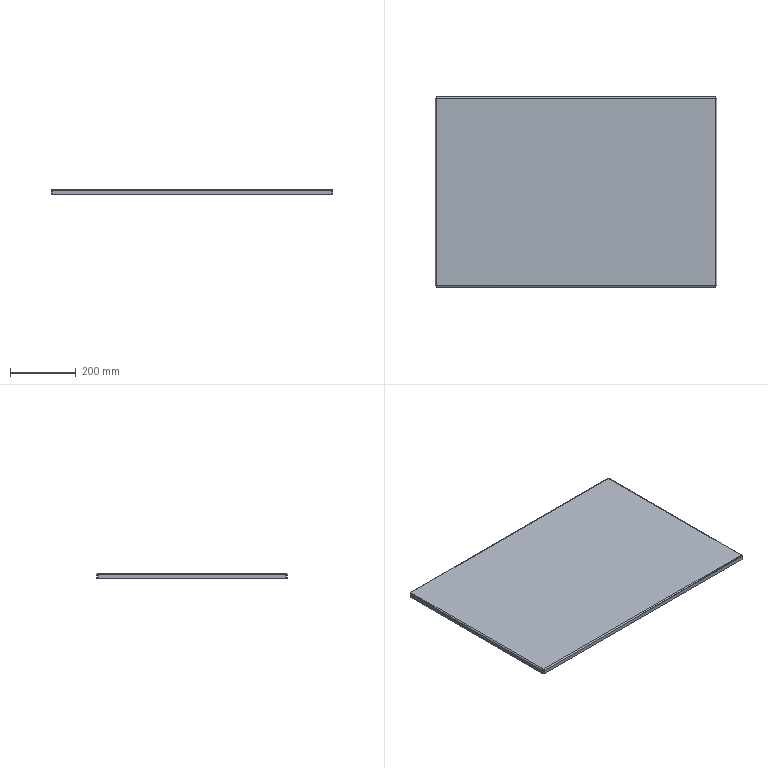Part | STEP file | MYT-A01-P36 | 1 solid | 38 faces | box 860 x 580 x 15 mm | volume 1590637 mm3 | plane 22 | spline 8 | cylinder 8 | commonest cylinder face diameters 1.473 x4 7.473 x4
STEP:
#1=CARTESIAN_POINT('',(-426.263,-286.263,-3.));
#2=VERTEX_POINT('',#1);
#3=CARTESIAN_POINT('',(426.263,-286.263,-3.));
#4=VERTEX_POINT('',#3);
#5=CARTESIAN_POINT('',(-426.293,-286.263,-3.));
#6=DIRECTION('',(1.,0.,0.));
#7=VECTOR('',#6,1000.);
#8=LINE('',#5,#7);
#9=EDGE_CURVE('',#2,#4,#8,.T.);
#10=ORIENTED_EDGE('',*,*,#9,.F.);
#11=CARTESIAN_POINT('',(-426.263,286.263,-3.));
#12=VERTEX_POINT('',#11);
#13=CARTESIAN_POINT('',(-426.263,286.293,-3.));
#14=DIRECTION('',(0.,-1.,0.));
#15=VECTOR('',#14,1000.);
#16=LINE('',#13,#15);
#17=EDGE_CURVE('',#12,#2,#16,.T.);
#18=ORIENTED_EDGE('',*,*,#17,.F.);
#19=CARTESIAN_POINT('',(426.263,286.263,-3.));
#20=VERTEX_POINT('',#19);
#21=CARTESIAN_POINT('',(426.293,286.263,-3.));
#22=DIRECTION('',(-1.,0.,0.));
#23=VECTOR('',#22,1000.);
#24=LINE('',#21,#23);
#25=EDGE_CURVE('',#20,#12,#24,.T.);
#26=ORIENTED_EDGE('',*,*,#25,.F.);
#27=CARTESIAN_POINT('',(426.263,-286.293,-3.));
#28=DIRECTION('',(0.,1.,0.));
#29=VECTOR('',#28,1000.);
#30=LINE('',#27,#29);
#31=EDGE_CURVE('',#4,#20,#30,.T.);
#32=ORIENTED_EDGE('',*,*,#31,.F.);
#33=EDGE_LOOP('',(#10,#18,#26,#32));
#34=FACE_OUTER_BOUND('',#33,.T.);
#35=CARTESIAN_POINT('',(0.,0.,-3.));
#36=DIRECTION('',(0.,0.,1.));
#37=DIRECTION('',(1.,0.,0.));
#38=AXIS2_PLACEMENT_3D('',#35,#36,#37);
#39=PLANE('',#38);
#40=ADVANCED_FACE('',(#34),#39,.F.);
#41=CARTESIAN_POINT('',(-426.263,286.263,0.));
#42=VERTEX_POINT('',#41);
#43=CARTESIAN_POINT('',(-426.263,-286.263,0.));
#44=VERTEX_POINT('',#43);
#45=CARTESIAN_POINT('',(-426.263,286.293,0.));
#46=DIRECTION('',(0.,-1.,0.));
#47=VECTOR('',#46,1000.);
#48=LINE('',#45,#47);
#49=EDGE_CURVE('',#42,#44,#48,.T.);
#50=ORIENTED_EDGE('',*,*,#49,.T.);
#51=CARTESIAN_POINT('',(426.263,-286.263,0.));
#52=VERTEX_POINT('',#51);
#53=CARTESIAN_POINT('',(-426.293,-286.263,0.));
#54=DIRECTION('',(1.,0.,0.));
#55=VECTOR('',#54,1000.);
#56=LINE('',#53,#55);
#57=EDGE_CURVE('',#44,#52,#56,.T.);
#58=ORIENTED_EDGE('',*,*,#57,.T.);
#59=CARTESIAN_POINT('',(426.263,286.263,0.));
#60=VERTEX_POINT('',#59);
#61=CARTESIAN_POINT('',(426.263,-286.293,0.));
#62=DIRECTION('',(0.,1.,0.));
#63=VECTOR('',#62,1000.);
#64=LINE('',#61,#63);
#65=EDGE_CURVE('',#52,#60,#64,.T.);
#66=ORIENTED_EDGE('',*,*,#65,.T.);
#67=CARTESIAN_POINT('',(426.293,286.263,0.));
#68=DIRECTION('',(-1.,0.,0.));
#69=VECTOR('',#68,1000.);
#70=LINE('',#67,#69);
#71=EDGE_CURVE('',#60,#42,#70,.T.);
#72=ORIENTED_EDGE('',*,*,#71,.T.);
#73=EDGE_LOOP('',(#50,#58,#66,#72));
#74=FACE_OUTER_BOUND('',#73,.T.);
#75=CARTESIAN_POINT('',(0.,0.,0.));
#76=DIRECTION('',(0.,0.,1.));
#77=DIRECTION('',(1.,0.,0.));
#78=AXIS2_PLACEMENT_3D('',#75,#76,#77);
#79=PLANE('',#78);
#80=ADVANCED_FACE('',(#74),#79,.T.);
#81=CARTESIAN_POINT('',(430.,286.293,-3.737));
#82=VERTEX_POINT('',#81);
#83=CARTESIAN_POINT('',(427.,286.293,-3.737));
#84=VERTEX_POINT('',#83);
#85=CARTESIAN_POINT('',(427.,286.293,-3.737));
#86=DIRECTION('',(-1.,0.,0.));
#87=VECTOR('',#86,1000.);
#88=LINE('',#85,#87);
#89=EDGE_CURVE('',#82,#84,#88,.T.);
#90=ORIENTED_EDGE('',*,*,#89,.T.);
#91=CARTESIAN_POINT('',(426.263,286.263,-3.));
#92=CARTESIAN_POINT('',(426.456,286.268,-3.));
#93=CARTESIAN_POINT('',(426.648,286.273,-3.079));
#94=CARTESIAN_POINT('',(426.921,286.283,-3.352));
#95=CARTESIAN_POINT('',(427.,286.288,-3.544));
#96=CARTESIAN_POINT('',(427.,286.293,-3.737));
#97=B_SPLINE_CURVE_WITH_KNOTS('',3,(#91,#92,#93,#94,#95,#96),.UNSPECIFIED.,.F.,.F.,(4,2,4),(0.,0.5,1.),.UNSPECIFIED.);
#98=EDGE_CURVE('',#20,#84,#97,.T.);
#99=ORIENTED_EDGE('',*,*,#98,.F.);
#100=CARTESIAN_POINT('',(426.263,286.263,-3.));
#101=DIRECTION('',(0.,0.,1.));
#102=VECTOR('',#101,1000.);
#103=LINE('',#100,#102);
#104=EDGE_CURVE('',#20,#60,#103,.T.);
#105=ORIENTED_EDGE('',*,*,#104,.T.);
#106=CARTESIAN_POINT('',(426.263,286.263,0.));
#107=CARTESIAN_POINT('',(426.753,286.266,0.));
#108=CARTESIAN_POINT('',(427.241,286.268,-0.09725));
#109=CARTESIAN_POINT('',(428.145,286.273,-0.4716));
#110=CARTESIAN_POINT('',(428.56,286.276,-0.7486));
#111=CARTESIAN_POINT('',(429.251,286.281,-1.44));
#112=CARTESIAN_POINT('',(429.528,286.283,-1.855));
#113=CARTESIAN_POINT('',(429.903,286.288,-2.759));
#114=CARTESIAN_POINT('',(430.,286.29,-3.247));
#115=CARTESIAN_POINT('',(430.,286.293,-3.737));
#116=B_SPLINE_CURVE_WITH_KNOTS('',3,(#106,#107,#108,#109,#110,#111,#112,#113,#114,#115),.UNSPECIFIED.,.F.,.F.,(4,2,2,2,4),(0.,0.25,0.5,0.75,1.),.UNSPECIFIED.);
#117=EDGE_CURVE('',#60,#82,#116,.T.);
#118=ORIENTED_EDGE('',*,*,#117,.T.);
#119=EDGE_LOOP('',(#90,#99,#105,#118));
#120=FACE_OUTER_BOUND('',#119,.T.);
#121=CARTESIAN_POINT('',(426.263,286.263,0.03));
#122=CARTESIAN_POINT('',(426.757,286.266,0.03));
#123=CARTESIAN_POINT('',(427.249,286.268,-0.06803));
#124=CARTESIAN_POINT('',(428.16,286.273,-0.4454));
#125=CARTESIAN_POINT('',(428.578,286.276,-0.7246));
#126=CARTESIAN_POINT('',(429.275,286.281,-1.422));
#127=CARTESIAN_POINT('',(429.555,286.283,-1.84));
#128=CARTESIAN_POINT('',(429.932,286.288,-2.751));
#129=CARTESIAN_POINT('',(430.03,286.29,-3.243));
#130=CARTESIAN_POINT('',(430.03,286.293,-3.737));
#131=CARTESIAN_POINT('',(426.263,286.263,0.));
#132=CARTESIAN_POINT('',(426.753,286.266,0.));
#133=CARTESIAN_POINT('',(427.241,286.268,-0.09725));
#134=CARTESIAN_POINT('',(428.145,286.273,-0.4716));
#135=CARTESIAN_POINT('',(428.56,286.276,-0.7486));
#136=CARTESIAN_POINT('',(429.251,286.281,-1.44));
#137=CARTESIAN_POINT('',(429.528,286.283,-1.855));
#138=CARTESIAN_POINT('',(429.903,286.288,-2.759));
#139=CARTESIAN_POINT('',(430.,286.29,-3.247));
#140=CARTESIAN_POINT('',(430.,286.293,-3.737));
#141=CARTESIAN_POINT('',(426.263,286.263,-3.));
#142=CARTESIAN_POINT('',(426.36,286.266,-3.));
#143=CARTESIAN_POINT('',(426.456,286.268,-3.019));
#144=CARTESIAN_POINT('',(426.634,286.273,-3.093));
#145=CARTESIAN_POINT('',(426.716,286.276,-3.148));
#146=CARTESIAN_POINT('',(426.852,286.281,-3.284));
#147=CARTESIAN_POINT('',(426.907,286.283,-3.366));
#148=CARTESIAN_POINT('',(426.981,286.288,-3.544));
#149=CARTESIAN_POINT('',(427.,286.29,-3.64));
#150=CARTESIAN_POINT('',(427.,286.293,-3.737));
#151=CARTESIAN_POINT('',(426.263,286.263,-3.03));
#152=CARTESIAN_POINT('',(426.356,286.266,-3.03));
#153=CARTESIAN_POINT('',(426.448,286.268,-3.049));
#154=CARTESIAN_POINT('',(426.619,286.273,-3.119));
#155=CARTESIAN_POINT('',(426.697,286.276,-3.172));
#156=CARTESIAN_POINT('',(426.828,286.281,-3.303));
#157=CARTESIAN_POINT('',(426.881,286.283,-3.381));
#158=CARTESIAN_POINT('',(426.951,286.288,-3.552));
#159=CARTESIAN_POINT('',(426.97,286.29,-3.644));
#160=CARTESIAN_POINT('',(426.97,286.293,-3.737));
#161=B_SPLINE_SURFACE_WITH_KNOTS('',1,3,((#121,#122,#123,#124,#125,#126,#127,#128,#129,#130),(#131,#132,#133,#134,#135,#136,#137,#138,#139,#140),(#141,#142,#143,#144,#145,#146,#147,#148,#149,#150),(#151,#152,#153,#154,#155,#156,#157,#158,#159,#160)),.UNSPECIFIED.,.F.,.F.,.F.,(2,1,1,2),(4,2,2,2,4),(-0.01,0.,1.,1.01),(0.,0.25,0.5,0.75,1.),.UNSPECIFIED.);
#162=ADVANCED_FACE('',(#120),#161,.F.);
#163=CARTESIAN_POINT('',(427.,-286.293,-3.737));
#164=VERTEX_POINT('',#163);
#165=CARTESIAN_POINT('',(427.,-286.293,-3.737));
#166=CARTESIAN_POINT('',(427.,-286.288,-3.544));
#167=CARTESIAN_POINT('',(426.921,-286.283,-3.352));
#168=CARTESIAN_POINT('',(426.648,-286.273,-3.079));
#169=CARTESIAN_POINT('',(426.456,-286.268,-3.));
#170=CARTESIAN_POINT('',(426.263,-286.263,-3.));
#171=B_SPLINE_CURVE_WITH_KNOTS('',3,(#165,#166,#167,#168,#169,#170),.UNSPECIFIED.,.F.,.F.,(4,2,4),(0.,0.5,1.),.UNSPECIFIED.);
#172=EDGE_CURVE('',#164,#4,#171,.T.);
#173=ORIENTED_EDGE('',*,*,#172,.F.);
#174=CARTESIAN_POINT('',(430.,-286.293,-3.737));
#175=VERTEX_POINT('',#174);
#176=CARTESIAN_POINT('',(427.,-286.293,-3.737));
#177=DIRECTION('',(-1.,0.,0.));
#178=VECTOR('',#177,1000.);
#179=LINE('',#176,#178);
#180=EDGE_CURVE('',#175,#164,#179,.T.);
#181=ORIENTED_EDGE('',*,*,#180,.F.);
#182=CARTESIAN_POINT('',(430.,-286.293,-3.737));
#183=CARTESIAN_POINT('',(430.,-286.29,-3.247));
#184=CARTESIAN_POINT('',(429.903,-286.288,-2.759));
#185=CARTESIAN_POINT('',(429.528,-286.283,-1.855));
#186=CARTESIAN_POINT('',(429.251,-286.281,-1.44));
#187=CARTESIAN_POINT('',(428.56,-286.276,-0.7486));
#188=CARTESIAN_POINT('',(428.145,-286.273,-0.4716));
#189=CARTESIAN_POINT('',(427.241,-286.268,-0.09725));
#190=CARTESIAN_POINT('',(426.753,-286.266,0.));
#191=CARTESIAN_POINT('',(426.263,-286.263,0.));
#192=B_SPLINE_CURVE_WITH_KNOTS('',3,(#182,#183,#184,#185,#186,#187,#188,#189,#190,#191),.UNSPECIFIED.,.F.,.F.,(4,2,2,2,4),(0.,0.25,0.5,0.75,1.),.UNSPECIFIED.);
#193=EDGE_CURVE('',#175,#52,#192,.T.);
#194=ORIENTED_EDGE('',*,*,#193,.T.);
#195=CARTESIAN_POINT('',(426.263,-286.263,-3.));
#196=DIRECTION('',(0.,0.,1.));
#197=VECTOR('',#196,1000.);
#198=LINE('',#195,#197);
#199=EDGE_CURVE('',#4,#52,#198,.T.);
#200=ORIENTED_EDGE('',*,*,#199,.F.);
#201=EDGE_LOOP('',(#173,#181,#194,#200));
#202=FACE_OUTER_BOUND('',#201,.T.);
#203=CARTESIAN_POINT('',(430.03,-286.293,-3.737));
#204=CARTESIAN_POINT('',(430.03,-286.29,-3.243));
#205=CARTESIAN_POINT('',(429.932,-286.288,-2.751));
#206=CARTESIAN_POINT('',(429.555,-286.283,-1.84));
#207=CARTESIAN_POINT('',(429.275,-286.281,-1.422));
#208=CARTESIAN_POINT('',(428.578,-286.276,-0.7246));
#209=CARTESIAN_POINT('',(428.16,-286.273,-0.4454));
#210=CARTESIAN_POINT('',(427.249,-286.268,-0.06803));
#211=CARTESIAN_POINT('',(426.757,-286.266,0.03));
#212=CARTESIAN_POINT('',(426.263,-286.263,0.03));
#213=CARTESIAN_POINT('',(430.,-286.293,-3.737));
#214=CARTESIAN_POINT('',(430.,-286.29,-3.247));
#215=CARTESIAN_POINT('',(429.903,-286.288,-2.759));
#216=CARTESIAN_POINT('',(429.528,-286.283,-1.855));
#217=CARTESIAN_POINT('',(429.251,-286.281,-1.44));
#218=CARTESIAN_POINT('',(428.56,-286.276,-0.7486));
#219=CARTESIAN_POINT('',(428.145,-286.273,-0.4716));
#220=CARTESIAN_POINT('',(427.241,-286.268,-0.09725));
#221=CARTESIAN_POINT('',(426.753,-286.266,0.));
#222=CARTESIAN_POINT('',(426.263,-286.263,0.));
#223=CARTESIAN_POINT('',(427.,-286.293,-3.737));
#224=CARTESIAN_POINT('',(427.,-286.29,-3.64));
#225=CARTESIAN_POINT('',(426.981,-286.288,-3.544));
#226=CARTESIAN_POINT('',(426.907,-286.283,-3.366));
#227=CARTESIAN_POINT('',(426.852,-286.281,-3.284));
#228=CARTESIAN_POINT('',(426.716,-286.276,-3.148));
#229=CARTESIAN_POINT('',(426.634,-286.273,-3.093));
#230=CARTESIAN_POINT('',(426.456,-286.268,-3.019));
#231=CARTESIAN_POINT('',(426.36,-286.266,-3.));
#232=CARTESIAN_POINT('',(426.263,-286.263,-3.));
#233=CARTESIAN_POINT('',(426.97,-286.293,-3.737));
#234=CARTESIAN_POINT('',(426.97,-286.29,-3.644));
#235=CARTESIAN_POINT('',(426.951,-286.288,-3.552));
#236=CARTESIAN_POINT('',(426.881,-286.283,-3.381));
#237=CARTESIAN_POINT('',(426.828,-286.281,-3.303));
#238=CARTESIAN_POINT('',(426.697,-286.276,-3.172));
#239=CARTESIAN_POINT('',(426.619,-286.273,-3.119));
#240=CARTESIAN_POINT('',(426.448,-286.268,-3.049));
#241=CARTESIAN_POINT('',(426.356,-286.266,-3.03));
#242=CARTESIAN_POINT('',(426.263,-286.263,-3.03));
#243=B_SPLINE_SURFACE_WITH_KNOTS('',1,3,((#203,#204,#205,#206,#207,#208,#209,#210,#211,#212),(#213,#214,#215,#216,#217,#218,#219,#220,#221,#222),(#223,#224,#225,#226,#227,#228,#229,#230,#231,#232),(#233,#234,#235,#236,#237,#238,#239,#240,#241,#242)),.UNSPECIFIED.,.F.,.F.,.F.,(2,1,1,2),(4,2,2,2,4),(-0.01,0.,1.,1.01),(0.,0.25,0.5,0.75,1.),.UNSPECIFIED.);
#244=ADVANCED_FACE('',(#202),#243,.F.);
#245=ORIENTED_EDGE('',*,*,#65,.F.);
#246=ORIENTED_EDGE('',*,*,#193,.F.);
#247=CARTESIAN_POINT('',(430.,290.,-3.737));
#248=DIRECTION('',(0.,1.,0.));
#249=VECTOR('',#248,1000.);
#250=LINE('',#247,#249);
#251=EDGE_CURVE('',#175,#82,#250,.T.);
#252=ORIENTED_EDGE('',*,*,#251,.T.);
#253=ORIENTED_EDGE('',*,*,#117,.F.);
#254=EDGE_LOOP('',(#245,#246,#252,#253));
#255=FACE_OUTER_BOUND('',#254,.T.);
#256=CARTESIAN_POINT('',(426.263,-286.293,-3.737));
#257=DIRECTION('',(0.,-1.,0.));
#258=DIRECTION('',(1.,0.,0.));
#259=AXIS2_PLACEMENT_3D('',#256,#257,#258);
#260=CYLINDRICAL_SURFACE('',#259,3.737);
#261=ADVANCED_FACE('',(#255),#260,.T.);
#262=ORIENTED_EDGE('',*,*,#31,.T.);
#263=ORIENTED_EDGE('',*,*,#98,.T.);
#264=CARTESIAN_POINT('',(427.,290.,-3.737));
#265=DIRECTION('',(0.,-1.,0.));
#266=VECTOR('',#265,1000.);
#267=LINE('',#264,#266);
#268=EDGE_CURVE('',#84,#164,#267,.T.);
#269=ORIENTED_EDGE('',*,*,#268,.T.);
#270=ORIENTED_EDGE('',*,*,#172,.T.);
#271=EDGE_LOOP('',(#262,#263,#269,#270));
#272=FACE_OUTER_BOUND('',#271,.T.);
#273=CARTESIAN_POINT('',(426.263,-286.293,-3.737));
#274=DIRECTION('',(0.,-1.,0.));
#275=DIRECTION('',(1.,0.,0.));
#276=AXIS2_PLACEMENT_3D('',#273,#274,#275);
#277=CYLINDRICAL_SURFACE('',#276,0.7366);
#278=ADVANCED_FACE('',(#272),#277,.F.);
#279=CARTESIAN_POINT('',(430.,286.293,-15.));
#280=VERTEX_POINT('',#279);
#281=CARTESIAN_POINT('',(430.,286.293,-3.));
#282=DIRECTION('',(0.,0.,-1.));
#283=VECTOR('',#282,1000.);
#284=LINE('',#281,#283);
#285=EDGE_CURVE('',#82,#280,#284,.T.);
#286=ORIENTED_EDGE('',*,*,#285,.T.);
#287=CARTESIAN_POINT('',(427.,286.293,-15.));
#288=VERTEX_POINT('',#287);
#289=CARTESIAN_POINT('',(427.,286.293,-15.));
#290=DIRECTION('',(-1.,0.,0.));
#291=VECTOR('',#290,1000.);
#292=LINE('',#289,#291);
#293=EDGE_CURVE('',#280,#288,#292,.T.);
#294=ORIENTED_EDGE('',*,*,#293,.T.);
#295=CARTESIAN_POINT('',(427.,286.293,0.));
#296=DIRECTION('',(0.,0.,-1.));
#297=VECTOR('',#296,1000.);
#298=LINE('',#295,#297);
#299=EDGE_CURVE('',#84,#288,#298,.T.);
#300=ORIENTED_EDGE('',*,*,#299,.F.);
#301=ORIENTED_EDGE('',*,*,#89,.F.);
#302=EDGE_LOOP('',(#286,#294,#300,#301));
#303=FACE_OUTER_BOUND('',#302,.T.);
#304=CARTESIAN_POINT('',(427.,286.293,-3.));
#305=DIRECTION('',(0.,1.,0.));
#306=DIRECTION('',(0.,0.,1.));
#307=AXIS2_PLACEMENT_3D('',#304,#305,#306);
#308=PLANE('',#307);
#309=ADVANCED_FACE('',(#303),#308,.T.);
#310=ORIENTED_EDGE('',*,*,#285,.F.);
#311=ORIENTED_EDGE('',*,*,#251,.F.);
#312=CARTESIAN_POINT('',(430.,-286.293,-15.));
#313=VERTEX_POINT('',#312);
#314=CARTESIAN_POINT('',(430.,-286.293,0.));
#315=DIRECTION('',(0.,0.,-1.));
#316=VECTOR('',#315,1000.);
#317=LINE('',#314,#316);
#318=EDGE_CURVE('',#175,#313,#317,.T.);
#319=ORIENTED_EDGE('',*,*,#318,.T.);
#320=CARTESIAN_POINT('',(430.,0.,-15.));
#321=DIRECTION('',(0.,1.,0.));
#322=VECTOR('',#321,1000.);
#323=LINE('',#320,#322);
#324=EDGE_CURVE('',#313,#280,#323,.T.);
#325=ORIENTED_EDGE('',*,*,#324,.T.);
#326=EDGE_LOOP('',(#310,#311,#319,#325));
#327=FACE_OUTER_BOUND('',#326,.T.);
#328=CARTESIAN_POINT('',(430.,0.,0.));
#329=DIRECTION('',(-1.,0.,0.));
#330=DIRECTION('',(0.,0.,1.));
#331=AXIS2_PLACEMENT_3D('',#328,#329,#330);
#332=PLANE('',#331);
#333=ADVANCED_FACE('',(#327),#332,.F.);
#334=ORIENTED_EDGE('',*,*,#268,.F.);
#335=ORIENTED_EDGE('',*,*,#299,.T.);
#336=CARTESIAN_POINT('',(427.,-286.293,-15.));
#337=VERTEX_POINT('',#336);
#338=CARTESIAN_POINT('',(427.,290.,-15.));
#339=DIRECTION('',(0.,1.,0.));
#340=VECTOR('',#339,1000.);
#341=LINE('',#338,#340);
#342=EDGE_CURVE('',#337,#288,#341,.T.);
#343=ORIENTED_EDGE('',*,*,#342,.F.);
#344=CARTESIAN_POINT('',(427.,-286.293,-3.));
#345=DIRECTION('',(0.,0.,-1.));
#346=VECTOR('',#345,1000.);
#347=LINE('',#344,#346);
#348=EDGE_CURVE('',#164,#337,#347,.T.);
#349=ORIENTED_EDGE('',*,*,#348,.F.);
#350=EDGE_LOOP('',(#334,#335,#343,#349));
#351=FACE_OUTER_BOUND('',#350,.T.);
#352=CARTESIAN_POINT('',(427.,0.,0.));
#353=DIRECTION('',(-1.,0.,0.));
#354=DIRECTION('',(0.,0.,1.));
#355=AXIS2_PLACEMENT_3D('',#352,#353,#354);
#356=PLANE('',#355);
#357=ADVANCED_FACE('',(#351),#356,.T.);
#358=ORIENTED_EDGE('',*,*,#293,.F.);
#359=ORIENTED_EDGE('',*,*,#324,.F.);
#360=CARTESIAN_POINT('',(430.,-286.293,-15.));
#361=DIRECTION('',(-1.,0.,0.));
#362=VECTOR('',#361,1000.);
#363=LINE('',#360,#362);
#364=EDGE_CURVE('',#313,#337,#363,.T.);
#365=ORIENTED_EDGE('',*,*,#364,.T.);
#366=ORIENTED_EDGE('',*,*,#342,.T.);
#367=EDGE_LOOP('',(#358,#359,#365,#366));
#368=FACE_OUTER_BOUND('',#367,.T.);
#369=CARTESIAN_POINT('',(430.,290.,-15.));
#370=DIRECTION('',(0.,0.,1.));
#371=DIRECTION('',(1.,0.,0.));
#372=AXIS2_PLACEMENT_3D('',#369,#370,#371);
#373=PLANE('',#372);
#374=ADVANCED_FACE('',(#368),#373,.F.);
#375=ORIENTED_EDGE('',*,*,#364,.F.);
#376=ORIENTED_EDGE('',*,*,#318,.F.);
#377=ORIENTED_EDGE('',*,*,#180,.T.);
#378=ORIENTED_EDGE('',*,*,#348,.T.);
#379=EDGE_LOOP('',(#375,#376,#377,#378));
#380=FACE_OUTER_BOUND('',#379,.T.);
#381=CARTESIAN_POINT('',(427.,-286.293,-3.));
#382=DIRECTION('',(0.,1.,0.));
#383=DIRECTION('',(0.,0.,1.));
#384=AXIS2_PLACEMENT_3D('',#381,#382,#383);
#385=PLANE('',#384);
#386=ADVANCED_FACE('',(#380),#385,.F.);
#387=CARTESIAN_POINT('',(-426.293,290.,-3.737));
#388=VERTEX_POINT('',#387);
#389=CARTESIAN_POINT('',(-426.293,287.,-3.737));
#390=VERTEX_POINT('',#389);
#391=CARTESIAN_POINT('',(-426.293,287.,-3.737));
#392=DIRECTION('',(0.,-1.,0.));
#393=VECTOR('',#392,1000.);
#394=LINE('',#391,#393);
#395=EDGE_CURVE('',#388,#390,#394,.T.);
#396=ORIENTED_EDGE('',*,*,#395,.T.);
#397=CARTESIAN_POINT('',(-426.263,286.263,-3.));
#398=CARTESIAN_POINT('',(-426.268,286.456,-3.));
#399=CARTESIAN_POINT('',(-426.273,286.648,-3.079));
#400=CARTESIAN_POINT('',(-426.283,286.921,-3.352));
#401=CARTESIAN_POINT('',(-426.288,287.,-3.544));
#402=CARTESIAN_POINT('',(-426.293,287.,-3.737));
#403=B_SPLINE_CURVE_WITH_KNOTS('',3,(#397,#398,#399,#400,#401,#402),.UNSPECIFIED.,.F.,.F.,(4,2,4),(0.,0.5,1.),.UNSPECIFIED.);
#404=EDGE_CURVE('',#12,#390,#403,.T.);
#405=ORIENTED_EDGE('',*,*,#404,.F.);
#406=CARTESIAN_POINT('',(-426.263,286.263,-3.));
#407=DIRECTION('',(0.,0.,1.));
#408=VECTOR('',#407,1000.);
#409=LINE('',#406,#408);
#410=EDGE_CURVE('',#12,#42,#409,.T.);
#411=ORIENTED_EDGE('',*,*,#410,.T.);
#412=CARTESIAN_POINT('',(-426.263,286.263,0.));
#413=CARTESIAN_POINT('',(-426.266,286.753,0.));
#414=CARTESIAN_POINT('',(-426.268,287.241,-0.09725));
#415=CARTESIAN_POINT('',(-426.273,288.145,-0.4716));
#416=CARTESIAN_POINT('',(-426.276,288.56,-0.7486));
#417=CARTESIAN_POINT('',(-426.281,289.251,-1.44));
#418=CARTESIAN_POINT('',(-426.283,289.528,-1.855));
#419=CARTESIAN_POINT('',(-426.288,289.903,-2.759));
#420=CARTESIAN_POINT('',(-426.29,290.,-3.247));
#421=CARTESIAN_POINT('',(-426.293,290.,-3.737));
#422=B_SPLINE_CURVE_WITH_KNOTS('',3,(#412,#413,#414,#415,#416,#417,#418,#419,#420,#421),.UNSPECIFIED.,.F.,.F.,(4,2,2,2,4),(0.,0.25,0.5,0.75,1.),.UNSPECIFIED.);
#423=EDGE_CURVE('',#42,#388,#422,.T.);
#424=ORIENTED_EDGE('',*,*,#423,.T.);
#425=EDGE_LOOP('',(#396,#405,#411,#424));
#426=FACE_OUTER_BOUND('',#425,.T.);
#427=CARTESIAN_POINT('',(-426.263,286.263,0.03));
#428=CARTESIAN_POINT('',(-426.266,286.757,0.03));
#429=CARTESIAN_POINT('',(-426.268,287.249,-0.06803));
#430=CARTESIAN_POINT('',(-426.273,288.16,-0.4454));
#431=CARTESIAN_POINT('',(-426.276,288.578,-0.7246));
#432=CARTESIAN_POINT('',(-426.281,289.275,-1.422));
#433=CARTESIAN_POINT('',(-426.283,289.555,-1.84));
#434=CARTESIAN_POINT('',(-426.288,289.932,-2.751));
#435=CARTESIAN_POINT('',(-426.29,290.03,-3.243));
#436=CARTESIAN_POINT('',(-426.293,290.03,-3.737));
#437=CARTESIAN_POINT('',(-426.263,286.263,0.));
#438=CARTESIAN_POINT('',(-426.266,286.753,0.));
#439=CARTESIAN_POINT('',(-426.268,287.241,-0.09725));
#440=CARTESIAN_POINT('',(-426.273,288.145,-0.4716));
#441=CARTESIAN_POINT('',(-426.276,288.56,-0.7486));
#442=CARTESIAN_POINT('',(-426.281,289.251,-1.44));
#443=CARTESIAN_POINT('',(-426.283,289.528,-1.855));
#444=CARTESIAN_POINT('',(-426.288,289.903,-2.759));
#445=CARTESIAN_POINT('',(-426.29,290.,-3.247));
#446=CARTESIAN_POINT('',(-426.293,290.,-3.737));
#447=CARTESIAN_POINT('',(-426.263,286.263,-3.));
#448=CARTESIAN_POINT('',(-426.266,286.36,-3.));
#449=CARTESIAN_POINT('',(-426.268,286.456,-3.019));
#450=CARTESIAN_POINT('',(-426.273,286.634,-3.093));
#451=CARTESIAN_POINT('',(-426.276,286.716,-3.148));
#452=CARTESIAN_POINT('',(-426.281,286.852,-3.284));
#453=CARTESIAN_POINT('',(-426.283,286.907,-3.366));
#454=CARTESIAN_POINT('',(-426.288,286.981,-3.544));
#455=CARTESIAN_POINT('',(-426.29,287.,-3.64));
#456=CARTESIAN_POINT('',(-426.293,287.,-3.737));
#457=CARTESIAN_POINT('',(-426.263,286.263,-3.03));
#458=CARTESIAN_POINT('',(-426.266,286.356,-3.03));
#459=CARTESIAN_POINT('',(-426.268,286.448,-3.049));
#460=CARTESIAN_POINT('',(-426.273,286.619,-3.119));
#461=CARTESIAN_POINT('',(-426.276,286.697,-3.172));
#462=CARTESIAN_POINT('',(-426.281,286.828,-3.303));
#463=CARTESIAN_POINT('',(-426.283,286.881,-3.381));
#464=CARTESIAN_POINT('',(-426.288,286.951,-3.552));
#465=CARTESIAN_POINT('',(-426.29,286.97,-3.644));
#466=CARTESIAN_POINT('',(-426.293,286.97,-3.737));
#467=B_SPLINE_SURFACE_WITH_KNOTS('',1,3,((#427,#428,#429,#430,#431,#432,#433,#434,#435,#436),(#437,#438,#439,#440,#441,#442,#443,#444,#445,#446),(#447,#448,#449,#450,#451,#452,#453,#454,#455,#456),(#457,#458,#459,#460,#461,#462,#463,#464,#465,#466)),.UNSPECIFIED.,.F.,.F.,.F.,(2,1,1,2),(4,2,2,2,4),(-0.01,0.,1.,1.01),(0.,0.25,0.5,0.75,1.),.UNSPECIFIED.);
#468=ADVANCED_FACE('',(#426),#467,.F.);
#469=CARTESIAN_POINT('',(426.293,287.,-3.737));
#470=VERTEX_POINT('',#469);
#471=CARTESIAN_POINT('',(426.293,287.,-3.737));
#472=CARTESIAN_POINT('',(426.288,287.,-3.544));
#473=CARTESIAN_POINT('',(426.283,286.921,-3.352));
#474=CARTESIAN_POINT('',(426.273,286.648,-3.079));
#475=CARTESIAN_POINT('',(426.268,286.456,-3.));
#476=CARTESIAN_POINT('',(426.263,286.263,-3.));
#477=B_SPLINE_CURVE_WITH_KNOTS('',3,(#471,#472,#473,#474,#475,#476),.UNSPECIFIED.,.F.,.F.,(4,2,4),(0.,0.5,1.),.UNSPECIFIED.);
#478=EDGE_CURVE('',#470,#20,#477,.T.);
#479=ORIENTED_EDGE('',*,*,#478,.F.);
#480=CARTESIAN_POINT('',(426.293,290.,-3.737));
#481=VERTEX_POINT('',#480);
#482=CARTESIAN_POINT('',(426.293,287.,-3.737));
#483=DIRECTION('',(0.,-1.,0.));
#484=VECTOR('',#483,1000.);
#485=LINE('',#482,#484);
#486=EDGE_CURVE('',#481,#470,#485,.T.);
#487=ORIENTED_EDGE('',*,*,#486,.F.);
#488=CARTESIAN_POINT('',(426.293,290.,-3.737));
#489=CARTESIAN_POINT('',(426.29,290.,-3.247));
#490=CARTESIAN_POINT('',(426.288,289.903,-2.759));
#491=CARTESIAN_POINT('',(426.283,289.528,-1.855));
#492=CARTESIAN_POINT('',(426.281,289.251,-1.44));
#493=CARTESIAN_POINT('',(426.276,288.56,-0.7486));
#494=CARTESIAN_POINT('',(426.273,288.145,-0.4716));
#495=CARTESIAN_POINT('',(426.268,287.241,-0.09725));
#496=CARTESIAN_POINT('',(426.266,286.753,0.));
#497=CARTESIAN_POINT('',(426.263,286.263,0.));
#498=B_SPLINE_CURVE_WITH_KNOTS('',3,(#488,#489,#490,#491,#492,#493,#494,#495,#496,#497),.UNSPECIFIED.,.F.,.F.,(4,2,2,2,4),(0.,0.25,0.5,0.75,1.),.UNSPECIFIED.);
#499=EDGE_CURVE('',#481,#60,#498,.T.);
#500=ORIENTED_EDGE('',*,*,#499,.T.);
#501=ORIENTED_EDGE('',*,*,#104,.F.);
#502=EDGE_LOOP('',(#479,#487,#500,#501));
#503=FACE_OUTER_BOUND('',#502,.T.);
#504=CARTESIAN_POINT('',(426.293,290.03,-3.737));
#505=CARTESIAN_POINT('',(426.29,290.03,-3.243));
#506=CARTESIAN_POINT('',(426.288,289.932,-2.751));
#507=CARTESIAN_POINT('',(426.283,289.555,-1.84));
#508=CARTESIAN_POINT('',(426.281,289.275,-1.422));
#509=CARTESIAN_POINT('',(426.276,288.578,-0.7246));
#510=CARTESIAN_POINT('',(426.273,288.16,-0.4454));
#511=CARTESIAN_POINT('',(426.268,287.249,-0.06803));
#512=CARTESIAN_POINT('',(426.266,286.757,0.03));
#513=CARTESIAN_POINT('',(426.263,286.263,0.03));
#514=CARTESIAN_POINT('',(426.293,290.,-3.737));
#515=CARTESIAN_POINT('',(426.29,290.,-3.247));
#516=CARTESIAN_POINT('',(426.288,289.903,-2.759));
#517=CARTESIAN_POINT('',(426.283,289.528,-1.855));
#518=CARTESIAN_POINT('',(426.281,289.251,-1.44));
#519=CARTESIAN_POINT('',(426.276,288.56,-0.7486));
#520=CARTESIAN_POINT('',(426.273,288.145,-0.4716));
#521=CARTESIAN_POINT('',(426.268,287.241,-0.09725));
#522=CARTESIAN_POINT('',(426.266,286.753,0.));
#523=CARTESIAN_POINT('',(426.263,286.263,0.));
#524=CARTESIAN_POINT('',(426.293,287.,-3.737));
#525=CARTESIAN_POINT('',(426.29,287.,-3.64));
#526=CARTESIAN_POINT('',(426.288,286.981,-3.544));
#527=CARTESIAN_POINT('',(426.283,286.907,-3.366));
#528=CARTESIAN_POINT('',(426.281,286.852,-3.284));
#529=CARTESIAN_POINT('',(426.276,286.716,-3.148));
#530=CARTESIAN_POINT('',(426.273,286.634,-3.093));
#531=CARTESIAN_POINT('',(426.268,286.456,-3.019));
#532=CARTESIAN_POINT('',(426.266,286.36,-3.));
#533=CARTESIAN_POINT('',(426.263,286.263,-3.));
#534=CARTESIAN_POINT('',(426.293,286.97,-3.737));
#535=CARTESIAN_POINT('',(426.29,286.97,-3.644));
#536=CARTESIAN_POINT('',(426.288,286.951,-3.552));
#537=CARTESIAN_POINT('',(426.283,286.881,-3.381));
#538=CARTESIAN_POINT('',(426.281,286.828,-3.303));
#539=CARTESIAN_POINT('',(426.276,286.697,-3.172));
#540=CARTESIAN_POINT('',(426.273,286.619,-3.119));
#541=CARTESIAN_POINT('',(426.268,286.448,-3.049));
#542=CARTESIAN_POINT('',(426.266,286.356,-3.03));
#543=CARTESIAN_POINT('',(426.263,286.263,-3.03));
#544=B_SPLINE_SURFACE_WITH_KNOTS('',1,3,((#504,#505,#506,#507,#508,#509,#510,#511,#512,#513),(#514,#515,#516,#517,#518,#519,#520,#521,#522,#523),(#524,#525,#526,#527,#528,#529,#530,#531,#532,#533),(#534,#535,#536,#537,#538,#539,#540,#541,#542,#543)),.UNSPECIFIED.,.F.,.F.,.F.,(2,1,1,2),(4,2,2,2,4),(-0.01,0.,1.,1.01),(0.,0.25,0.5,0.75,1.),.UNSPECIFIED.);
#545=ADVANCED_FACE('',(#503),#544,.F.);
#546=ORIENTED_EDGE('',*,*,#71,.F.);
#547=ORIENTED_EDGE('',*,*,#499,.F.);
#548=CARTESIAN_POINT('',(-430.,290.,-3.737));
#549=DIRECTION('',(-1.,0.,0.));
#550=VECTOR('',#549,1000.);
#551=LINE('',#548,#550);
#552=EDGE_CURVE('',#481,#388,#551,.T.);
#553=ORIENTED_EDGE('',*,*,#552,.T.);
#554=ORIENTED_EDGE('',*,*,#423,.F.);
#555=EDGE_LOOP('',(#546,#547,#553,#554));
#556=FACE_OUTER_BOUND('',#555,.T.);
#557=CARTESIAN_POINT('',(426.293,286.263,-3.737));
#558=DIRECTION('',(1.,0.,0.));
#559=DIRECTION('',(0.,1.,0.));
#560=AXIS2_PLACEMENT_3D('',#557,#558,#559);
#561=CYLINDRICAL_SURFACE('',#560,3.737);
#562=ADVANCED_FACE('',(#556),#561,.T.);
#563=ORIENTED_EDGE('',*,*,#25,.T.);
#564=ORIENTED_EDGE('',*,*,#404,.T.);
#565=CARTESIAN_POINT('',(-430.,287.,-3.737));
#566=DIRECTION('',(1.,0.,0.));
#567=VECTOR('',#566,1000.);
#568=LINE('',#565,#567);
#569=EDGE_CURVE('',#390,#470,#568,.T.);
#570=ORIENTED_EDGE('',*,*,#569,.T.);
#571=ORIENTED_EDGE('',*,*,#478,.T.);
#572=EDGE_LOOP('',(#563,#564,#570,#571));
#573=FACE_OUTER_BOUND('',#572,.T.);
#574=CARTESIAN_POINT('',(426.293,286.263,-3.737));
#575=DIRECTION('',(1.,0.,0.));
#576=DIRECTION('',(0.,1.,0.));
#577=AXIS2_PLACEMENT_3D('',#574,#575,#576);
#578=CYLINDRICAL_SURFACE('',#577,0.7366);
#579=ADVANCED_FACE('',(#573),#578,.F.);
#580=CARTESIAN_POINT('',(-426.293,290.,-15.));
#581=VERTEX_POINT('',#580);
#582=CARTESIAN_POINT('',(-426.293,290.,-3.));
#583=DIRECTION('',(0.,0.,-1.));
#584=VECTOR('',#583,1000.);
#585=LINE('',#582,#584);
#586=EDGE_CURVE('',#388,#581,#585,.T.);
#587=ORIENTED_EDGE('',*,*,#586,.T.);
#588=CARTESIAN_POINT('',(-426.293,287.,-15.));
#589=VERTEX_POINT('',#588);
#590=CARTESIAN_POINT('',(-426.293,287.,-15.));
#591=DIRECTION('',(0.,-1.,0.));
#592=VECTOR('',#591,1000.);
#593=LINE('',#590,#592);
#594=EDGE_CURVE('',#581,#589,#593,.T.);
#595=ORIENTED_EDGE('',*,*,#594,.T.);
#596=CARTESIAN_POINT('',(-426.293,287.,0.));
#597=DIRECTION('',(0.,0.,-1.));
#598=VECTOR('',#597,1000.);
#599=LINE('',#596,#598);
#600=EDGE_CURVE('',#390,#589,#599,.T.);
#601=ORIENTED_EDGE('',*,*,#600,.F.);
#602=ORIENTED_EDGE('',*,*,#395,.F.);
#603=EDGE_LOOP('',(#587,#595,#601,#602));
#604=FACE_OUTER_BOUND('',#603,.T.);
#605=CARTESIAN_POINT('',(-426.293,287.,-3.));
#606=DIRECTION('',(-1.,0.,0.));
#607=DIRECTION('',(0.,0.,1.));
#608=AXIS2_PLACEMENT_3D('',#605,#606,#607);
#609=PLANE('',#608);
#610=ADVANCED_FACE('',(#604),#609,.T.);
#611=ORIENTED_EDGE('',*,*,#586,.F.);
#612=ORIENTED_EDGE('',*,*,#552,.F.);
#613=CARTESIAN_POINT('',(426.293,290.,-15.));
#614=VERTEX_POINT('',#613);
#615=CARTESIAN_POINT('',(426.293,290.,0.));
#616=DIRECTION('',(0.,0.,-1.));
#617=VECTOR('',#616,1000.);
#618=LINE('',#615,#617);
#619=EDGE_CURVE('',#481,#614,#618,.T.);
#620=ORIENTED_EDGE('',*,*,#619,.T.);
#621=CARTESIAN_POINT('',(0.,290.,-15.));
#622=DIRECTION('',(-1.,0.,0.));
#623=VECTOR('',#622,1000.);
#624=LINE('',#621,#623);
#625=EDGE_CURVE('',#614,#581,#624,.T.);
#626=ORIENTED_EDGE('',*,*,#625,.T.);
#627=EDGE_LOOP('',(#611,#612,#620,#626));
#628=FACE_OUTER_BOUND('',#627,.T.);
#629=CARTESIAN_POINT('',(0.,290.,0.));
#630=DIRECTION('',(0.,-1.,0.));
#631=DIRECTION('',(0.,0.,-1.));
#632=AXIS2_PLACEMENT_3D('',#629,#630,#631);
#633=PLANE('',#632);
#634=ADVANCED_FACE('',(#628),#633,.F.);
#635=ORIENTED_EDGE('',*,*,#569,.F.);
#636=ORIENTED_EDGE('',*,*,#600,.T.);
#637=CARTESIAN_POINT('',(426.293,287.,-15.));
#638=VERTEX_POINT('',#637);
#639=CARTESIAN_POINT('',(-430.,287.,-15.));
#640=DIRECTION('',(-1.,0.,0.));
#641=VECTOR('',#640,1000.);
#642=LINE('',#639,#641);
#643=EDGE_CURVE('',#638,#589,#642,.T.);
#644=ORIENTED_EDGE('',*,*,#643,.F.);
#645=CARTESIAN_POINT('',(426.293,287.,-3.));
#646=DIRECTION('',(0.,0.,-1.));
#647=VECTOR('',#646,1000.);
#648=LINE('',#645,#647);
#649=EDGE_CURVE('',#470,#638,#648,.T.);
#650=ORIENTED_EDGE('',*,*,#649,.F.);
#651=EDGE_LOOP('',(#635,#636,#644,#650));
#652=FACE_OUTER_BOUND('',#651,.T.);
#653=CARTESIAN_POINT('',(0.,287.,0.));
#654=DIRECTION('',(0.,-1.,0.));
#655=DIRECTION('',(0.,0.,-1.));
#656=AXIS2_PLACEMENT_3D('',#653,#654,#655);
#657=PLANE('',#656);
#658=ADVANCED_FACE('',(#652),#657,.T.);
#659=ORIENTED_EDGE('',*,*,#594,.F.);
#660=ORIENTED_EDGE('',*,*,#625,.F.);
#661=CARTESIAN_POINT('',(426.293,290.,-15.));
#662=DIRECTION('',(0.,-1.,0.));
#663=VECTOR('',#662,1000.);
#664=LINE('',#661,#663);
#665=EDGE_CURVE('',#614,#638,#664,.T.);
#666=ORIENTED_EDGE('',*,*,#665,.T.);
#667=ORIENTED_EDGE('',*,*,#643,.T.);
#668=EDGE_LOOP('',(#659,#660,#666,#667));
#669=FACE_OUTER_BOUND('',#668,.T.);
#670=CARTESIAN_POINT('',(-430.,290.,-15.));
#671=DIRECTION('',(0.,0.,1.));
#672=DIRECTION('',(0.,-1.,0.));
#673=AXIS2_PLACEMENT_3D('',#670,#671,#672);
#674=PLANE('',#673);
#675=ADVANCED_FACE('',(#669),#674,.F.);
#676=ORIENTED_EDGE('',*,*,#665,.F.);
#677=ORIENTED_EDGE('',*,*,#619,.F.);
#678=ORIENTED_EDGE('',*,*,#486,.T.);
#679=ORIENTED_EDGE('',*,*,#649,.T.);
#680=EDGE_LOOP('',(#676,#677,#678,#679));
#681=FACE_OUTER_BOUND('',#680,.T.);
#682=CARTESIAN_POINT('',(426.293,287.,-3.));
#683=DIRECTION('',(-1.,0.,0.));
#684=DIRECTION('',(0.,0.,1.));
#685=AXIS2_PLACEMENT_3D('',#682,#683,#684);
#686=PLANE('',#685);
#687=ADVANCED_FACE('',(#681),#686,.F.);
#688=CARTESIAN_POINT('',(-430.,-286.293,-3.737));
#689=VERTEX_POINT('',#688);
#690=CARTESIAN_POINT('',(-427.,-286.293,-3.737));
#691=VERTEX_POINT('',#690);
#692=CARTESIAN_POINT('',(-427.,-286.293,-3.737));
#693=DIRECTION('',(1.,0.,0.));
#694=VECTOR('',#693,1000.);
#695=LINE('',#692,#694);
#696=EDGE_CURVE('',#689,#691,#695,.T.);
#697=ORIENTED_EDGE('',*,*,#696,.T.);
#698=CARTESIAN_POINT('',(-426.263,-286.263,-3.));
#699=CARTESIAN_POINT('',(-426.456,-286.268,-3.));
#700=CARTESIAN_POINT('',(-426.648,-286.273,-3.079));
#701=CARTESIAN_POINT('',(-426.921,-286.283,-3.352));
#702=CARTESIAN_POINT('',(-427.,-286.288,-3.544));
#703=CARTESIAN_POINT('',(-427.,-286.293,-3.737));
#704=B_SPLINE_CURVE_WITH_KNOTS('',3,(#698,#699,#700,#701,#702,#703),.UNSPECIFIED.,.F.,.F.,(4,2,4),(0.,0.5,1.),.UNSPECIFIED.);
#705=EDGE_CURVE('',#2,#691,#704,.T.);
#706=ORIENTED_EDGE('',*,*,#705,.F.);
#707=CARTESIAN_POINT('',(-426.263,-286.263,-3.));
#708=DIRECTION('',(0.,0.,1.));
#709=VECTOR('',#708,1000.);
#710=LINE('',#707,#709);
#711=EDGE_CURVE('',#2,#44,#710,.T.);
#712=ORIENTED_EDGE('',*,*,#711,.T.);
#713=CARTESIAN_POINT('',(-426.263,-286.263,0.));
#714=CARTESIAN_POINT('',(-426.753,-286.266,0.));
#715=CARTESIAN_POINT('',(-427.241,-286.268,-0.09725));
#716=CARTESIAN_POINT('',(-428.145,-286.273,-0.4716));
#717=CARTESIAN_POINT('',(-428.56,-286.276,-0.7486));
#718=CARTESIAN_POINT('',(-429.251,-286.281,-1.44));
#719=CARTESIAN_POINT('',(-429.528,-286.283,-1.855));
#720=CARTESIAN_POINT('',(-429.903,-286.288,-2.759));
#721=CARTESIAN_POINT('',(-430.,-286.29,-3.247));
#722=CARTESIAN_POINT('',(-430.,-286.293,-3.737));
#723=B_SPLINE_CURVE_WITH_KNOTS('',3,(#713,#714,#715,#716,#717,#718,#719,#720,#721,#722),.UNSPECIFIED.,.F.,.F.,(4,2,2,2,4),(0.,0.25,0.5,0.75,1.),.UNSPECIFIED.);
#724=EDGE_CURVE('',#44,#689,#723,.T.);
#725=ORIENTED_EDGE('',*,*,#724,.T.);
#726=EDGE_LOOP('',(#697,#706,#712,#725));
#727=FACE_OUTER_BOUND('',#726,.T.);
#728=CARTESIAN_POINT('',(-426.263,-286.263,0.03));
#729=CARTESIAN_POINT('',(-426.757,-286.266,0.03));
#730=CARTESIAN_POINT('',(-427.249,-286.268,-0.06803));
#731=CARTESIAN_POINT('',(-428.16,-286.273,-0.4454));
#732=CARTESIAN_POINT('',(-428.578,-286.276,-0.7246));
#733=CARTESIAN_POINT('',(-429.275,-286.281,-1.422));
#734=CARTESIAN_POINT('',(-429.555,-286.283,-1.84));
#735=CARTESIAN_POINT('',(-429.932,-286.288,-2.751));
#736=CARTESIAN_POINT('',(-430.03,-286.29,-3.243));
#737=CARTESIAN_POINT('',(-430.03,-286.293,-3.737));
#738=CARTESIAN_POINT('',(-426.263,-286.263,0.));
#739=CARTESIAN_POINT('',(-426.753,-286.266,0.));
#740=CARTESIAN_POINT('',(-427.241,-286.268,-0.09725));
#741=CARTESIAN_POINT('',(-428.145,-286.273,-0.4716));
#742=CARTESIAN_POINT('',(-428.56,-286.276,-0.7486));
#743=CARTESIAN_POINT('',(-429.251,-286.281,-1.44));
#744=CARTESIAN_POINT('',(-429.528,-286.283,-1.855));
#745=CARTESIAN_POINT('',(-429.903,-286.288,-2.759));
#746=CARTESIAN_POINT('',(-430.,-286.29,-3.247));
#747=CARTESIAN_POINT('',(-430.,-286.293,-3.737));
#748=CARTESIAN_POINT('',(-426.263,-286.263,-3.));
#749=CARTESIAN_POINT('',(-426.36,-286.266,-3.));
#750=CARTESIAN_POINT('',(-426.456,-286.268,-3.019));
#751=CARTESIAN_POINT('',(-426.634,-286.273,-3.093));
#752=CARTESIAN_POINT('',(-426.716,-286.276,-3.148));
#753=CARTESIAN_POINT('',(-426.852,-286.281,-3.284));
#754=CARTESIAN_POINT('',(-426.907,-286.283,-3.366));
#755=CARTESIAN_POINT('',(-426.981,-286.288,-3.544));
#756=CARTESIAN_POINT('',(-427.,-286.29,-3.64));
#757=CARTESIAN_POINT('',(-427.,-286.293,-3.737));
#758=CARTESIAN_POINT('',(-426.263,-286.263,-3.03));
#759=CARTESIAN_POINT('',(-426.356,-286.266,-3.03));
#760=CARTESIAN_POINT('',(-426.448,-286.268,-3.049));
#761=CARTESIAN_POINT('',(-426.619,-286.273,-3.119));
#762=CARTESIAN_POINT('',(-426.697,-286.276,-3.172));
#763=CARTESIAN_POINT('',(-426.828,-286.281,-3.303));
#764=CARTESIAN_POINT('',(-426.881,-286.283,-3.381));
#765=CARTESIAN_POINT('',(-426.951,-286.288,-3.552));
#766=CARTESIAN_POINT('',(-426.97,-286.29,-3.644));
#767=CARTESIAN_POINT('',(-426.97,-286.293,-3.737));
#768=B_SPLINE_SURFACE_WITH_KNOTS('',1,3,((#728,#729,#730,#731,#732,#733,#734,#735,#736,#737),(#738,#739,#740,#741,#742,#743,#744,#745,#746,#747),(#748,#749,#750,#751,#752,#753,#754,#755,#756,#757),(#758,#759,#760,#761,#762,#763,#764,#765,#766,#767)),.UNSPECIFIED.,.F.,.F.,.F.,(2,1,1,2),(4,2,2,2,4),(-0.01,0.,1.,1.01),(0.,0.25,0.5,0.75,1.),.UNSPECIFIED.);
#769=ADVANCED_FACE('',(#727),#768,.F.);
#770=CARTESIAN_POINT('',(-427.,286.293,-3.737));
#771=VERTEX_POINT('',#770);
#772=CARTESIAN_POINT('',(-427.,286.293,-3.737));
#773=CARTESIAN_POINT('',(-427.,286.288,-3.544));
#774=CARTESIAN_POINT('',(-426.921,286.283,-3.352));
#775=CARTESIAN_POINT('',(-426.648,286.273,-3.079));
#776=CARTESIAN_POINT('',(-426.456,286.268,-3.));
#777=CARTESIAN_POINT('',(-426.263,286.263,-3.));
#778=B_SPLINE_CURVE_WITH_KNOTS('',3,(#772,#773,#774,#775,#776,#777),.UNSPECIFIED.,.F.,.F.,(4,2,4),(0.,0.5,1.),.UNSPECIFIED.);
#779=EDGE_CURVE('',#771,#12,#778,.T.);
#780=ORIENTED_EDGE('',*,*,#779,.F.);
#781=CARTESIAN_POINT('',(-430.,286.293,-3.737));
#782=VERTEX_POINT('',#781);
#783=CARTESIAN_POINT('',(-427.,286.293,-3.737));
#784=DIRECTION('',(1.,0.,0.));
#785=VECTOR('',#784,1000.);
#786=LINE('',#783,#785);
#787=EDGE_CURVE('',#782,#771,#786,.T.);
#788=ORIENTED_EDGE('',*,*,#787,.F.);
#789=CARTESIAN_POINT('',(-430.,286.293,-3.737));
#790=CARTESIAN_POINT('',(-430.,286.29,-3.247));
#791=CARTESIAN_POINT('',(-429.903,286.288,-2.759));
#792=CARTESIAN_POINT('',(-429.528,286.283,-1.855));
#793=CARTESIAN_POINT('',(-429.251,286.281,-1.44));
#794=CARTESIAN_POINT('',(-428.56,286.276,-0.7486));
#795=CARTESIAN_POINT('',(-428.145,286.273,-0.4716));
#796=CARTESIAN_POINT('',(-427.241,286.268,-0.09725));
#797=CARTESIAN_POINT('',(-426.753,286.266,0.));
#798=CARTESIAN_POINT('',(-426.263,286.263,0.));
#799=B_SPLINE_CURVE_WITH_KNOTS('',3,(#789,#790,#791,#792,#793,#794,#795,#796,#797,#798),.UNSPECIFIED.,.F.,.F.,(4,2,2,2,4),(0.,0.25,0.5,0.75,1.),.UNSPECIFIED.);
#800=EDGE_CURVE('',#782,#42,#799,.T.);
#801=ORIENTED_EDGE('',*,*,#800,.T.);
#802=ORIENTED_EDGE('',*,*,#410,.F.);
#803=EDGE_LOOP('',(#780,#788,#801,#802));
#804=FACE_OUTER_BOUND('',#803,.T.);
#805=CARTESIAN_POINT('',(-430.03,286.293,-3.737));
#806=CARTESIAN_POINT('',(-430.03,286.29,-3.243));
#807=CARTESIAN_POINT('',(-429.932,286.288,-2.751));
#808=CARTESIAN_POINT('',(-429.555,286.283,-1.84));
#809=CARTESIAN_POINT('',(-429.275,286.281,-1.422));
#810=CARTESIAN_POINT('',(-428.578,286.276,-0.7246));
#811=CARTESIAN_POINT('',(-428.16,286.273,-0.4454));
#812=CARTESIAN_POINT('',(-427.249,286.268,-0.06803));
#813=CARTESIAN_POINT('',(-426.757,286.266,0.03));
#814=CARTESIAN_POINT('',(-426.263,286.263,0.03));
#815=CARTESIAN_POINT('',(-430.,286.293,-3.737));
#816=CARTESIAN_POINT('',(-430.,286.29,-3.247));
#817=CARTESIAN_POINT('',(-429.903,286.288,-2.759));
#818=CARTESIAN_POINT('',(-429.528,286.283,-1.855));
#819=CARTESIAN_POINT('',(-429.251,286.281,-1.44));
#820=CARTESIAN_POINT('',(-428.56,286.276,-0.7486));
#821=CARTESIAN_POINT('',(-428.145,286.273,-0.4716));
#822=CARTESIAN_POINT('',(-427.241,286.268,-0.09725));
#823=CARTESIAN_POINT('',(-426.753,286.266,0.));
#824=CARTESIAN_POINT('',(-426.263,286.263,0.));
#825=CARTESIAN_POINT('',(-427.,286.293,-3.737));
#826=CARTESIAN_POINT('',(-427.,286.29,-3.64));
#827=CARTESIAN_POINT('',(-426.981,286.288,-3.544));
#828=CARTESIAN_POINT('',(-426.907,286.283,-3.366));
#829=CARTESIAN_POINT('',(-426.852,286.281,-3.284));
#830=CARTESIAN_POINT('',(-426.716,286.276,-3.148));
#831=CARTESIAN_POINT('',(-426.634,286.273,-3.093));
#832=CARTESIAN_POINT('',(-426.456,286.268,-3.019));
#833=CARTESIAN_POINT('',(-426.36,286.266,-3.));
#834=CARTESIAN_POINT('',(-426.263,286.263,-3.));
#835=CARTESIAN_POINT('',(-426.97,286.293,-3.737));
#836=CARTESIAN_POINT('',(-426.97,286.29,-3.644));
#837=CARTESIAN_POINT('',(-426.951,286.288,-3.552));
#838=CARTESIAN_POINT('',(-426.881,286.283,-3.381));
#839=CARTESIAN_POINT('',(-426.828,286.281,-3.303));
#840=CARTESIAN_POINT('',(-426.697,286.276,-3.172));
#841=CARTESIAN_POINT('',(-426.619,286.273,-3.119));
#842=CARTESIAN_POINT('',(-426.448,286.268,-3.049));
#843=CARTESIAN_POINT('',(-426.356,286.266,-3.03));
#844=CARTESIAN_POINT('',(-426.263,286.263,-3.03));
#845=B_SPLINE_SURFACE_WITH_KNOTS('',1,3,((#805,#806,#807,#808,#809,#810,#811,#812,#813,#814),(#815,#816,#817,#818,#819,#820,#821,#822,#823,#824),(#825,#826,#827,#828,#829,#830,#831,#832,#833,#834),(#835,#836,#837,#838,#839,#840,#841,#842,#843,#844)),.UNSPECIFIED.,.F.,.F.,.F.,(2,1,1,2),(4,2,2,2,4),(-0.01,0.,1.,1.01),(0.,0.25,0.5,0.75,1.),.UNSPECIFIED.);
#846=ADVANCED_FACE('',(#804),#845,.F.);
#847=ORIENTED_EDGE('',*,*,#49,.F.);
#848=ORIENTED_EDGE('',*,*,#800,.F.);
#849=CARTESIAN_POINT('',(-430.,-290.,-3.737));
#850=DIRECTION('',(0.,-1.,0.));
#851=VECTOR('',#850,1000.);
#852=LINE('',#849,#851);
#853=EDGE_CURVE('',#782,#689,#852,.T.);
#854=ORIENTED_EDGE('',*,*,#853,.T.);
#855=ORIENTED_EDGE('',*,*,#724,.F.);
#856=EDGE_LOOP('',(#847,#848,#854,#855));
#857=FACE_OUTER_BOUND('',#856,.T.);
#858=CARTESIAN_POINT('',(-426.263,286.293,-3.737));
#859=DIRECTION('',(0.,1.,0.));
#860=DIRECTION('',(-1.,0.,0.));
#861=AXIS2_PLACEMENT_3D('',#858,#859,#860);
#862=CYLINDRICAL_SURFACE('',#861,3.737);
#863=ADVANCED_FACE('',(#857),#862,.T.);
#864=ORIENTED_EDGE('',*,*,#17,.T.);
#865=ORIENTED_EDGE('',*,*,#705,.T.);
#866=CARTESIAN_POINT('',(-427.,-290.,-3.737));
#867=DIRECTION('',(0.,1.,0.));
#868=VECTOR('',#867,1000.);
#869=LINE('',#866,#868);
#870=EDGE_CURVE('',#691,#771,#869,.T.);
#871=ORIENTED_EDGE('',*,*,#870,.T.);
#872=ORIENTED_EDGE('',*,*,#779,.T.);
#873=EDGE_LOOP('',(#864,#865,#871,#872));
#874=FACE_OUTER_BOUND('',#873,.T.);
#875=CARTESIAN_POINT('',(-426.263,286.293,-3.737));
#876=DIRECTION('',(0.,1.,0.));
#877=DIRECTION('',(-1.,0.,0.));
#878=AXIS2_PLACEMENT_3D('',#875,#876,#877);
#879=CYLINDRICAL_SURFACE('',#878,0.7366);
#880=ADVANCED_FACE('',(#874),#879,.F.);
#881=CARTESIAN_POINT('',(-430.,-286.293,-15.));
#882=VERTEX_POINT('',#881);
#883=CARTESIAN_POINT('',(-430.,-286.293,-3.));
#884=DIRECTION('',(0.,0.,-1.));
#885=VECTOR('',#884,1000.);
#886=LINE('',#883,#885);
#887=EDGE_CURVE('',#689,#882,#886,.T.);
#888=ORIENTED_EDGE('',*,*,#887,.T.);
#889=CARTESIAN_POINT('',(-427.,-286.293,-15.));
#890=VERTEX_POINT('',#889);
#891=CARTESIAN_POINT('',(-427.,-286.293,-15.));
#892=DIRECTION('',(1.,0.,0.));
#893=VECTOR('',#892,1000.);
#894=LINE('',#891,#893);
#895=EDGE_CURVE('',#882,#890,#894,.T.);
#896=ORIENTED_EDGE('',*,*,#895,.T.);
#897=CARTESIAN_POINT('',(-427.,-286.293,0.));
#898=DIRECTION('',(0.,0.,-1.));
#899=VECTOR('',#898,1000.);
#900=LINE('',#897,#899);
#901=EDGE_CURVE('',#691,#890,#900,.T.);
#902=ORIENTED_EDGE('',*,*,#901,.F.);
#903=ORIENTED_EDGE('',*,*,#696,.F.);
#904=EDGE_LOOP('',(#888,#896,#902,#903));
#905=FACE_OUTER_BOUND('',#904,.T.);
#906=CARTESIAN_POINT('',(-427.,-286.293,-3.));
#907=DIRECTION('',(0.,-1.,0.));
#908=DIRECTION('',(0.,0.,-1.));
#909=AXIS2_PLACEMENT_3D('',#906,#907,#908);
#910=PLANE('',#909);
#911=ADVANCED_FACE('',(#905),#910,.T.);
#912=ORIENTED_EDGE('',*,*,#887,.F.);
#913=ORIENTED_EDGE('',*,*,#853,.F.);
#914=CARTESIAN_POINT('',(-430.,286.293,-15.));
#915=VERTEX_POINT('',#914);
#916=CARTESIAN_POINT('',(-430.,286.293,0.));
#917=DIRECTION('',(0.,0.,-1.));
#918=VECTOR('',#917,1000.);
#919=LINE('',#916,#918);
#920=EDGE_CURVE('',#782,#915,#919,.T.);
#921=ORIENTED_EDGE('',*,*,#920,.T.);
#922=CARTESIAN_POINT('',(-430.,0.,-15.));
#923=DIRECTION('',(0.,-1.,0.));
#924=VECTOR('',#923,1000.);
#925=LINE('',#922,#924);
#926=EDGE_CURVE('',#915,#882,#925,.T.);
#927=ORIENTED_EDGE('',*,*,#926,.T.);
#928=EDGE_LOOP('',(#912,#913,#921,#927));
#929=FACE_OUTER_BOUND('',#928,.T.);
#930=CARTESIAN_POINT('',(-430.,0.,0.));
#931=DIRECTION('',(1.,0.,0.));
#932=DIRECTION('',(0.,1.,0.));
#933=AXIS2_PLACEMENT_3D('',#930,#931,#932);
#934=PLANE('',#933);
#935=ADVANCED_FACE('',(#929),#934,.F.);
#936=ORIENTED_EDGE('',*,*,#870,.F.);
#937=ORIENTED_EDGE('',*,*,#901,.T.);
#938=CARTESIAN_POINT('',(-427.,286.293,-15.));
#939=VERTEX_POINT('',#938);
#940=CARTESIAN_POINT('',(-427.,-290.,-15.));
#941=DIRECTION('',(0.,-1.,0.));
#942=VECTOR('',#941,1000.);
#943=LINE('',#940,#942);
#944=EDGE_CURVE('',#939,#890,#943,.T.);
#945=ORIENTED_EDGE('',*,*,#944,.F.);
#946=CARTESIAN_POINT('',(-427.,286.293,-3.));
#947=DIRECTION('',(0.,0.,-1.));
#948=VECTOR('',#947,1000.);
#949=LINE('',#946,#948);
#950=EDGE_CURVE('',#771,#939,#949,.T.);
#951=ORIENTED_EDGE('',*,*,#950,.F.);
#952=EDGE_LOOP('',(#936,#937,#945,#951));
#953=FACE_OUTER_BOUND('',#952,.T.);
#954=CARTESIAN_POINT('',(-427.,0.,0.));
#955=DIRECTION('',(1.,0.,0.));
#956=DIRECTION('',(0.,1.,0.));
#957=AXIS2_PLACEMENT_3D('',#954,#955,#956);
#958=PLANE('',#957);
#959=ADVANCED_FACE('',(#953),#958,.T.);
#960=ORIENTED_EDGE('',*,*,#895,.F.);
#961=ORIENTED_EDGE('',*,*,#926,.F.);
#962=CARTESIAN_POINT('',(-430.,286.293,-15.));
#963=DIRECTION('',(1.,0.,0.));
#964=VECTOR('',#963,1000.);
#965=LINE('',#962,#964);
#966=EDGE_CURVE('',#915,#939,#965,.T.);
#967=ORIENTED_EDGE('',*,*,#966,.T.);
#968=ORIENTED_EDGE('',*,*,#944,.T.);
#969=EDGE_LOOP('',(#960,#961,#967,#968));
#970=FACE_OUTER_BOUND('',#969,.T.);
#971=CARTESIAN_POINT('',(-430.,-290.,-15.));
#972=DIRECTION('',(0.,0.,1.));
#973=DIRECTION('',(1.,0.,0.));
#974=AXIS2_PLACEMENT_3D('',#971,#972,#973);
#975=PLANE('',#974);
#976=ADVANCED_FACE('',(#970),#975,.F.);
#977=ORIENTED_EDGE('',*,*,#966,.F.);
#978=ORIENTED_EDGE('',*,*,#920,.F.);
#979=ORIENTED_EDGE('',*,*,#787,.T.);
#980=ORIENTED_EDGE('',*,*,#950,.T.);
#981=EDGE_LOOP('',(#977,#978,#979,#980));
#982=FACE_OUTER_BOUND('',#981,.T.);
#983=CARTESIAN_POINT('',(-427.,286.293,-3.));
#984=DIRECTION('',(0.,-1.,0.));
#985=DIRECTION('',(0.,0.,-1.));
#986=AXIS2_PLACEMENT_3D('',#983,#984,#985);
#987=PLANE('',#986);
#988=ADVANCED_FACE('',(#982),#987,.F.);
#989=CARTESIAN_POINT('',(426.293,-290.,-3.737));
#990=VERTEX_POINT('',#989);
#991=CARTESIAN_POINT('',(426.293,-287.,-3.737));
#992=VERTEX_POINT('',#991);
#993=CARTESIAN_POINT('',(426.293,-287.,-3.737));
#994=DIRECTION('',(0.,1.,0.));
#995=VECTOR('',#994,1000.);
#996=LINE('',#993,#995);
#997=EDGE_CURVE('',#990,#992,#996,.T.);
#998=ORIENTED_EDGE('',*,*,#997,.T.);
#999=CARTESIAN_POINT('',(426.263,-286.263,-3.));
#1000=CARTESIAN_POINT('',(426.268,-286.456,-3.));
#1001=CARTESIAN_POINT('',(426.273,-286.648,-3.079));
#1002=CARTESIAN_POINT('',(426.283,-286.921,-3.352));
#1003=CARTESIAN_POINT('',(426.288,-287.,-3.544));
#1004=CARTESIAN_POINT('',(426.293,-287.,-3.737));
#1005=B_SPLINE_CURVE_WITH_KNOTS('',3,(#999,#1000,#1001,#1002,#1003,#1004),.UNSPECIFIED.,.F.,.F.,(4,2,4),(0.,0.5,1.),.UNSPECIFIED.);
#1006=EDGE_CURVE('',#4,#992,#1005,.T.);
#1007=ORIENTED_EDGE('',*,*,#1006,.F.);
#1008=ORIENTED_EDGE('',*,*,#199,.T.);
#1009=CARTESIAN_POINT('',(426.263,-286.263,0.));
#1010=CARTESIAN_POINT('',(426.266,-286.753,0.));
#1011=CARTESIAN_POINT('',(426.268,-287.241,-0.09725));
#1012=CARTESIAN_POINT('',(426.273,-288.145,-0.4716));
#1013=CARTESIAN_POINT('',(426.276,-288.56,-0.7486));
#1014=CARTESIAN_POINT('',(426.281,-289.251,-1.44));
#1015=CARTESIAN_POINT('',(426.283,-289.528,-1.855));
#1016=CARTESIAN_POINT('',(426.288,-289.903,-2.759));
#1017=CARTESIAN_POINT('',(426.29,-290.,-3.247));
#1018=CARTESIAN_POINT('',(426.293,-290.,-3.737));
#1019=B_SPLINE_CURVE_WITH_KNOTS('',3,(#1009,#1010,#1011,#1012,#1013,#1014,#1015,#1016,#1017,#1018),.UNSPECIFIED.,.F.,.F.,(4,2,2,2,4),(0.,0.25,0.5,0.75,1.),.UNSPECIFIED.);
#1020=EDGE_CURVE('',#52,#990,#1019,.T.);
#1021=ORIENTED_EDGE('',*,*,#1020,.T.);
#1022=EDGE_LOOP('',(#998,#1007,#1008,#1021));
#1023=FACE_OUTER_BOUND('',#1022,.T.);
#1024=CARTESIAN_POINT('',(426.263,-286.263,0.03));
#1025=CARTESIAN_POINT('',(426.266,-286.757,0.03));
#1026=CARTESIAN_POINT('',(426.268,-287.249,-0.06803));
#1027=CARTESIAN_POINT('',(426.273,-288.16,-0.4454));
#1028=CARTESIAN_POINT('',(426.276,-288.578,-0.7246));
#1029=CARTESIAN_POINT('',(426.281,-289.275,-1.422));
#1030=CARTESIAN_POINT('',(426.283,-289.555,-1.84));
#1031=CARTESIAN_POINT('',(426.288,-289.932,-2.751));
#1032=CARTESIAN_POINT('',(426.29,-290.03,-3.243));
#1033=CARTESIAN_POINT('',(426.293,-290.03,-3.737));
#1034=CARTESIAN_POINT('',(426.263,-286.263,0.));
#1035=CARTESIAN_POINT('',(426.266,-286.753,0.));
#1036=CARTESIAN_POINT('',(426.268,-287.241,-0.09725));
#1037=CARTESIAN_POINT('',(426.273,-288.145,-0.4716));
#1038=CARTESIAN_POINT('',(426.276,-288.56,-0.7486));
#1039=CARTESIAN_POINT('',(426.281,-289.251,-1.44));
#1040=CARTESIAN_POINT('',(426.283,-289.528,-1.855));
#1041=CARTESIAN_POINT('',(426.288,-289.903,-2.759));
#1042=CARTESIAN_POINT('',(426.29,-290.,-3.247));
#1043=CARTESIAN_POINT('',(426.293,-290.,-3.737));
#1044=CARTESIAN_POINT('',(426.263,-286.263,-3.));
#1045=CARTESIAN_POINT('',(426.266,-286.36,-3.));
#1046=CARTESIAN_POINT('',(426.268,-286.456,-3.019));
#1047=CARTESIAN_POINT('',(426.273,-286.634,-3.093));
#1048=CARTESIAN_POINT('',(426.276,-286.716,-3.148));
#1049=CARTESIAN_POINT('',(426.281,-286.852,-3.284));
#1050=CARTESIAN_POINT('',(426.283,-286.907,-3.366));
#1051=CARTESIAN_POINT('',(426.288,-286.981,-3.544));
#1052=CARTESIAN_POINT('',(426.29,-287.,-3.64));
#1053=CARTESIAN_POINT('',(426.293,-287.,-3.737));
#1054=CARTESIAN_POINT('',(426.263,-286.263,-3.03));
#1055=CARTESIAN_POINT('',(426.266,-286.356,-3.03));
#1056=CARTESIAN_POINT('',(426.268,-286.448,-3.049));
#1057=CARTESIAN_POINT('',(426.273,-286.619,-3.119));
#1058=CARTESIAN_POINT('',(426.276,-286.697,-3.172));
#1059=CARTESIAN_POINT('',(426.281,-286.828,-3.303));
#1060=CARTESIAN_POINT('',(426.283,-286.881,-3.381));
#1061=CARTESIAN_POINT('',(426.288,-286.951,-3.552));
#1062=CARTESIAN_POINT('',(426.29,-286.97,-3.644));
#1063=CARTESIAN_POINT('',(426.293,-286.97,-3.737));
#1064=B_SPLINE_SURFACE_WITH_KNOTS('',1,3,((#1024,#1025,#1026,#1027,#1028,#1029,#1030,#1031,#1032,#1033),(#1034,#1035,#1036,#1037,#1038,#1039,#1040,#1041,#1042,#1043),(#1044,#1045,#1046,#1047,#1048,#1049,#1050,#1051,#1052,#1053),(#1054,#1055,#1056,#1057,#1058,#1059,#1060,#1061,#1062,#1063)),.UNSPECIFIED.,.F.,.F.,.F.,(2,1,1,2),(4,2,2,2,4),(-0.01,0.,1.,1.01),(0.,0.25,0.5,0.75,1.),.UNSPECIFIED.);
#1065=ADVANCED_FACE('',(#1023),#1064,.F.);
#1066=CARTESIAN_POINT('',(-426.293,-287.,-3.737));
#1067=VERTEX_POINT('',#1066);
#1068=CARTESIAN_POINT('',(-426.293,-287.,-3.737));
#1069=CARTESIAN_POINT('',(-426.288,-287.,-3.544));
#1070=CARTESIAN_POINT('',(-426.283,-286.921,-3.352));
#1071=CARTESIAN_POINT('',(-426.273,-286.648,-3.079));
#1072=CARTESIAN_POINT('',(-426.268,-286.456,-3.));
#1073=CARTESIAN_POINT('',(-426.263,-286.263,-3.));
#1074=B_SPLINE_CURVE_WITH_KNOTS('',3,(#1068,#1069,#1070,#1071,#1072,#1073),.UNSPECIFIED.,.F.,.F.,(4,2,4),(0.,0.5,1.),.UNSPECIFIED.);
#1075=EDGE_CURVE('',#1067,#2,#1074,.T.);
#1076=ORIENTED_EDGE('',*,*,#1075,.F.);
#1077=CARTESIAN_POINT('',(-426.293,-290.,-3.737));
#1078=VERTEX_POINT('',#1077);
#1079=CARTESIAN_POINT('',(-426.293,-287.,-3.737));
#1080=DIRECTION('',(0.,1.,0.));
#1081=VECTOR('',#1080,1000.);
#1082=LINE('',#1079,#1081);
#1083=EDGE_CURVE('',#1078,#1067,#1082,.T.);
#1084=ORIENTED_EDGE('',*,*,#1083,.F.);
#1085=CARTESIAN_POINT('',(-426.293,-290.,-3.737));
#1086=CARTESIAN_POINT('',(-426.29,-290.,-3.247));
#1087=CARTESIAN_POINT('',(-426.288,-289.903,-2.759));
#1088=CARTESIAN_POINT('',(-426.283,-289.528,-1.855));
#1089=CARTESIAN_POINT('',(-426.281,-289.251,-1.44));
#1090=CARTESIAN_POINT('',(-426.276,-288.56,-0.7486));
#1091=CARTESIAN_POINT('',(-426.273,-288.145,-0.4716));
#1092=CARTESIAN_POINT('',(-426.268,-287.241,-0.09725));
#1093=CARTESIAN_POINT('',(-426.266,-286.753,0.));
#1094=CARTESIAN_POINT('',(-426.263,-286.263,0.));
#1095=B_SPLINE_CURVE_WITH_KNOTS('',3,(#1085,#1086,#1087,#1088,#1089,#1090,#1091,#1092,#1093,#1094),.UNSPECIFIED.,.F.,.F.,(4,2,2,2,4),(0.,0.25,0.5,0.75,1.),.UNSPECIFIED.);
#1096=EDGE_CURVE('',#1078,#44,#1095,.T.);
#1097=ORIENTED_EDGE('',*,*,#1096,.T.);
#1098=ORIENTED_EDGE('',*,*,#711,.F.);
#1099=EDGE_LOOP('',(#1076,#1084,#1097,#1098));
#1100=FACE_OUTER_BOUND('',#1099,.T.);
#1101=CARTESIAN_POINT('',(-426.293,-290.03,-3.737));
#1102=CARTESIAN_POINT('',(-426.29,-290.03,-3.243));
#1103=CARTESIAN_POINT('',(-426.288,-289.932,-2.751));
#1104=CARTESIAN_POINT('',(-426.283,-289.555,-1.84));
#1105=CARTESIAN_POINT('',(-426.281,-289.275,-1.422));
#1106=CARTESIAN_POINT('',(-426.276,-288.578,-0.7246));
#1107=CARTESIAN_POINT('',(-426.273,-288.16,-0.4454));
#1108=CARTESIAN_POINT('',(-426.268,-287.249,-0.06803));
#1109=CARTESIAN_POINT('',(-426.266,-286.757,0.03));
#1110=CARTESIAN_POINT('',(-426.263,-286.263,0.03));
#1111=CARTESIAN_POINT('',(-426.293,-290.,-3.737));
#1112=CARTESIAN_POINT('',(-426.29,-290.,-3.247));
#1113=CARTESIAN_POINT('',(-426.288,-289.903,-2.759));
#1114=CARTESIAN_POINT('',(-426.283,-289.528,-1.855));
#1115=CARTESIAN_POINT('',(-426.281,-289.251,-1.44));
#1116=CARTESIAN_POINT('',(-426.276,-288.56,-0.7486));
#1117=CARTESIAN_POINT('',(-426.273,-288.145,-0.4716));
#1118=CARTESIAN_POINT('',(-426.268,-287.241,-0.09725));
#1119=CARTESIAN_POINT('',(-426.266,-286.753,0.));
#1120=CARTESIAN_POINT('',(-426.263,-286.263,0.));
#1121=CARTESIAN_POINT('',(-426.293,-287.,-3.737));
#1122=CARTESIAN_POINT('',(-426.29,-287.,-3.64));
#1123=CARTESIAN_POINT('',(-426.288,-286.981,-3.544));
#1124=CARTESIAN_POINT('',(-426.283,-286.907,-3.366));
#1125=CARTESIAN_POINT('',(-426.281,-286.852,-3.284));
#1126=CARTESIAN_POINT('',(-426.276,-286.716,-3.148));
#1127=CARTESIAN_POINT('',(-426.273,-286.634,-3.093));
#1128=CARTESIAN_POINT('',(-426.268,-286.456,-3.019));
#1129=CARTESIAN_POINT('',(-426.266,-286.36,-3.));
#1130=CARTESIAN_POINT('',(-426.263,-286.263,-3.));
#1131=CARTESIAN_POINT('',(-426.293,-286.97,-3.737));
#1132=CARTESIAN_POINT('',(-426.29,-286.97,-3.644));
#1133=CARTESIAN_POINT('',(-426.288,-286.951,-3.552));
#1134=CARTESIAN_POINT('',(-426.283,-286.881,-3.381));
#1135=CARTESIAN_POINT('',(-426.281,-286.828,-3.303));
#1136=CARTESIAN_POINT('',(-426.276,-286.697,-3.172));
#1137=CARTESIAN_POINT('',(-426.273,-286.619,-3.119));
#1138=CARTESIAN_POINT('',(-426.268,-286.448,-3.049));
#1139=CARTESIAN_POINT('',(-426.266,-286.356,-3.03));
#1140=CARTESIAN_POINT('',(-426.263,-286.263,-3.03));
#1141=B_SPLINE_SURFACE_WITH_KNOTS('',1,3,((#1101,#1102,#1103,#1104,#1105,#1106,#1107,#1108,#1109,#1110),(#1111,#1112,#1113,#1114,#1115,#1116,#1117,#1118,#1119,#1120),(#1121,#1122,#1123,#1124,#1125,#1126,#1127,#1128,#1129,#1130),(#1131,#1132,#1133,#1134,#1135,#1136,#1137,#1138,#1139,#1140)),.UNSPECIFIED.,.F.,.F.,.F.,(2,1,1,2),(4,2,2,2,4),(-0.01,0.,1.,1.01),(0.,0.25,0.5,0.75,1.),.UNSPECIFIED.);
#1142=ADVANCED_FACE('',(#1100),#1141,.F.);
#1143=ORIENTED_EDGE('',*,*,#57,.F.);
#1144=ORIENTED_EDGE('',*,*,#1096,.F.);
#1145=CARTESIAN_POINT('',(430.,-290.,-3.737));
#1146=DIRECTION('',(1.,0.,0.));
#1147=VECTOR('',#1146,1000.);
#1148=LINE('',#1145,#1147);
#1149=EDGE_CURVE('',#1078,#990,#1148,.T.);
#1150=ORIENTED_EDGE('',*,*,#1149,.T.);
#1151=ORIENTED_EDGE('',*,*,#1020,.F.);
#1152=EDGE_LOOP('',(#1143,#1144,#1150,#1151));
#1153=FACE_OUTER_BOUND('',#1152,.T.);
#1154=CARTESIAN_POINT('',(-426.293,-286.263,-3.737));
#1155=DIRECTION('',(-1.,0.,0.));
#1156=DIRECTION('',(0.,-1.,0.));
#1157=AXIS2_PLACEMENT_3D('',#1154,#1155,#1156);
#1158=CYLINDRICAL_SURFACE('',#1157,3.737);
#1159=ADVANCED_FACE('',(#1153),#1158,.T.);
#1160=ORIENTED_EDGE('',*,*,#9,.T.);
#1161=ORIENTED_EDGE('',*,*,#1006,.T.);
#1162=CARTESIAN_POINT('',(430.,-287.,-3.737));
#1163=DIRECTION('',(-1.,0.,0.));
#1164=VECTOR('',#1163,1000.);
#1165=LINE('',#1162,#1164);
#1166=EDGE_CURVE('',#992,#1067,#1165,.T.);
#1167=ORIENTED_EDGE('',*,*,#1166,.T.);
#1168=ORIENTED_EDGE('',*,*,#1075,.T.);
#1169=EDGE_LOOP('',(#1160,#1161,#1167,#1168));
#1170=FACE_OUTER_BOUND('',#1169,.T.);
#1171=CARTESIAN_POINT('',(-426.293,-286.263,-3.737));
#1172=DIRECTION('',(-1.,0.,0.));
#1173=DIRECTION('',(0.,-1.,0.));
#1174=AXIS2_PLACEMENT_3D('',#1171,#1172,#1173);
#1175=CYLINDRICAL_SURFACE('',#1174,0.7366);
#1176=ADVANCED_FACE('',(#1170),#1175,.F.);
#1177=CARTESIAN_POINT('',(426.293,-290.,-15.));
#1178=VERTEX_POINT('',#1177);
#1179=CARTESIAN_POINT('',(426.293,-290.,-3.));
#1180=DIRECTION('',(0.,0.,-1.));
#1181=VECTOR('',#1180,1000.);
#1182=LINE('',#1179,#1181);
#1183=EDGE_CURVE('',#990,#1178,#1182,.T.);
#1184=ORIENTED_EDGE('',*,*,#1183,.T.);
#1185=CARTESIAN_POINT('',(426.293,-287.,-15.));
#1186=VERTEX_POINT('',#1185);
#1187=CARTESIAN_POINT('',(426.293,-287.,-15.));
#1188=DIRECTION('',(0.,1.,0.));
#1189=VECTOR('',#1188,1000.);
#1190=LINE('',#1187,#1189);
#1191=EDGE_CURVE('',#1178,#1186,#1190,.T.);
#1192=ORIENTED_EDGE('',*,*,#1191,.T.);
#1193=CARTESIAN_POINT('',(426.293,-287.,0.));
#1194=DIRECTION('',(0.,0.,-1.));
#1195=VECTOR('',#1194,1000.);
#1196=LINE('',#1193,#1195);
#1197=EDGE_CURVE('',#992,#1186,#1196,.T.);
#1198=ORIENTED_EDGE('',*,*,#1197,.F.);
#1199=ORIENTED_EDGE('',*,*,#997,.F.);
#1200=EDGE_LOOP('',(#1184,#1192,#1198,#1199));
#1201=FACE_OUTER_BOUND('',#1200,.T.);
#1202=CARTESIAN_POINT('',(426.293,-287.,-3.));
#1203=DIRECTION('',(1.,0.,0.));
#1204=DIRECTION('',(0.,0.,-1.));
#1205=AXIS2_PLACEMENT_3D('',#1202,#1203,#1204);
#1206=PLANE('',#1205);
#1207=ADVANCED_FACE('',(#1201),#1206,.T.);
#1208=ORIENTED_EDGE('',*,*,#1183,.F.);
#1209=ORIENTED_EDGE('',*,*,#1149,.F.);
#1210=CARTESIAN_POINT('',(-426.293,-290.,-15.));
#1211=VERTEX_POINT('',#1210);
#1212=CARTESIAN_POINT('',(-426.293,-290.,0.));
#1213=DIRECTION('',(0.,0.,-1.));
#1214=VECTOR('',#1213,1000.);
#1215=LINE('',#1212,#1214);
#1216=EDGE_CURVE('',#1078,#1211,#1215,.T.);
#1217=ORIENTED_EDGE('',*,*,#1216,.T.);
#1218=CARTESIAN_POINT('',(0.,-290.,-15.));
#1219=DIRECTION('',(1.,0.,0.));
#1220=VECTOR('',#1219,1000.);
#1221=LINE('',#1218,#1220);
#1222=EDGE_CURVE('',#1211,#1178,#1221,.T.);
#1223=ORIENTED_EDGE('',*,*,#1222,.T.);
#1224=EDGE_LOOP('',(#1208,#1209,#1217,#1223));
#1225=FACE_OUTER_BOUND('',#1224,.T.);
#1226=CARTESIAN_POINT('',(0.,-290.,0.));
#1227=DIRECTION('',(0.,1.,0.));
#1228=DIRECTION('',(0.,0.,1.));
#1229=AXIS2_PLACEMENT_3D('',#1226,#1227,#1228);
#1230=PLANE('',#1229);
#1231=ADVANCED_FACE('',(#1225),#1230,.F.);
#1232=ORIENTED_EDGE('',*,*,#1166,.F.);
#1233=ORIENTED_EDGE('',*,*,#1197,.T.);
#1234=CARTESIAN_POINT('',(-426.293,-287.,-15.));
#1235=VERTEX_POINT('',#1234);
#1236=CARTESIAN_POINT('',(430.,-287.,-15.));
#1237=DIRECTION('',(1.,0.,0.));
#1238=VECTOR('',#1237,1000.);
#1239=LINE('',#1236,#1238);
#1240=EDGE_CURVE('',#1235,#1186,#1239,.T.);
#1241=ORIENTED_EDGE('',*,*,#1240,.F.);
#1242=CARTESIAN_POINT('',(-426.293,-287.,-3.));
#1243=DIRECTION('',(0.,0.,-1.));
#1244=VECTOR('',#1243,1000.);
#1245=LINE('',#1242,#1244);
#1246=EDGE_CURVE('',#1067,#1235,#1245,.T.);
#1247=ORIENTED_EDGE('',*,*,#1246,.F.);
#1248=EDGE_LOOP('',(#1232,#1233,#1241,#1247));
#1249=FACE_OUTER_BOUND('',#1248,.T.);
#1250=CARTESIAN_POINT('',(0.,-287.,0.));
#1251=DIRECTION('',(0.,1.,0.));
#1252=DIRECTION('',(0.,0.,1.));
#1253=AXIS2_PLACEMENT_3D('',#1250,#1251,#1252);
#1254=PLANE('',#1253);
#1255=ADVANCED_FACE('',(#1249),#1254,.T.);
#1256=ORIENTED_EDGE('',*,*,#1191,.F.);
#1257=ORIENTED_EDGE('',*,*,#1222,.F.);
#1258=CARTESIAN_POINT('',(-426.293,-290.,-15.));
#1259=DIRECTION('',(0.,1.,0.));
#1260=VECTOR('',#1259,1000.);
#1261=LINE('',#1258,#1260);
#1262=EDGE_CURVE('',#1211,#1235,#1261,.T.);
#1263=ORIENTED_EDGE('',*,*,#1262,.T.);
#1264=ORIENTED_EDGE('',*,*,#1240,.T.);
#1265=EDGE_LOOP('',(#1256,#1257,#1263,#1264));
#1266=FACE_OUTER_BOUND('',#1265,.T.);
#1267=CARTESIAN_POINT('',(430.,-290.,-15.));
#1268=DIRECTION('',(0.,0.,1.));
#1269=DIRECTION('',(0.,-1.,0.));
#1270=AXIS2_PLACEMENT_3D('',#1267,#1268,#1269);
#1271=PLANE('',#1270);
#1272=ADVANCED_FACE('',(#1266),#1271,.F.);
#1273=ORIENTED_EDGE('',*,*,#1262,.F.);
#1274=ORIENTED_EDGE('',*,*,#1216,.F.);
#1275=ORIENTED_EDGE('',*,*,#1083,.T.);
#1276=ORIENTED_EDGE('',*,*,#1246,.T.);
#1277=EDGE_LOOP('',(#1273,#1274,#1275,#1276));
#1278=FACE_OUTER_BOUND('',#1277,.T.);
#1279=CARTESIAN_POINT('',(-426.293,-287.,-3.));
#1280=DIRECTION('',(1.,0.,0.));
#1281=DIRECTION('',(0.,0.,-1.));
#1282=AXIS2_PLACEMENT_3D('',#1279,#1280,#1281);
#1283=PLANE('',#1282);
#1284=ADVANCED_FACE('',(#1278),#1283,.F.);
#1285=CLOSED_SHELL('',(#40,#80,#162,#244,#261,#278,#309,#333,#357,#374,#386,#468,#545,#562,#579,#610,#634,#658,#675,#687,#769,#846,#863,#880,#911,#935,#959,#976,#988,#1065,#1142,#1159,#1176,#1207,#1231,#1255,#1272,#1284));
#1286=MANIFOLD_SOLID_BREP('',#1285);
#1287=CARTESIAN_POINT('',(0.,0.,0.));
#1288=DIRECTION('',(0.,0.,1.));
#1289=DIRECTION('',(1.,0.,0.));
#1290=AXIS2_PLACEMENT_3D('',#1287,#1288,#1289);
#1291=(LENGTH_UNIT()NAMED_UNIT(*)SI_UNIT(.MILLI.,.METRE.));
#1292=UNCERTAINTY_MEASURE_WITH_UNIT(LENGTH_MEASURE(0.00001),#1291,'','');
#1293=(NAMED_UNIT(*)PLANE_ANGLE_UNIT()SI_UNIT($,.RADIAN.));
#1294=(NAMED_UNIT(*)SI_UNIT($,.STERADIAN.)SOLID_ANGLE_UNIT());
#1295=(GEOMETRIC_REPRESENTATION_CONTEXT(3)GLOBAL_UNCERTAINTY_ASSIGNED_CONTEXT((#1292))GLOBAL_UNIT_ASSIGNED_CONTEXT((#1291,#1293,#1294))REPRESENTATION_CONTEXT('',''));
#1296=ADVANCED_BREP_SHAPE_REPRESENTATION('',(#1286,#1290),#1295);